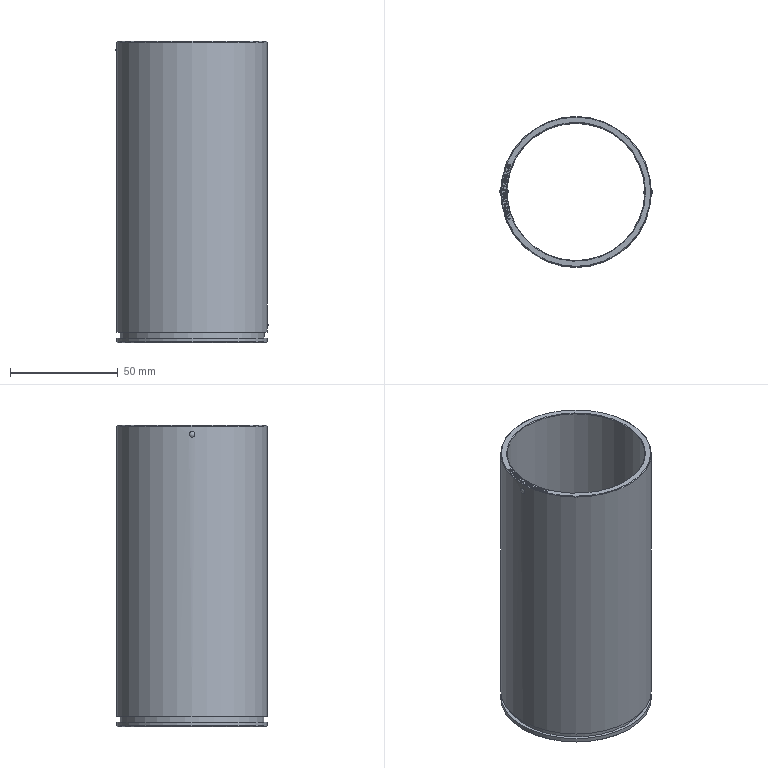Part | NX | features solid 2 | 1 solid | 260 faces | box 71 x 70 x 140 mm | volume 87516 mm3 | spline 138 | plane 110 | cone 4 | cylinder 4 | sphere 4 | commonest cylinder face diameters 70 x2 64 x1 67 x1